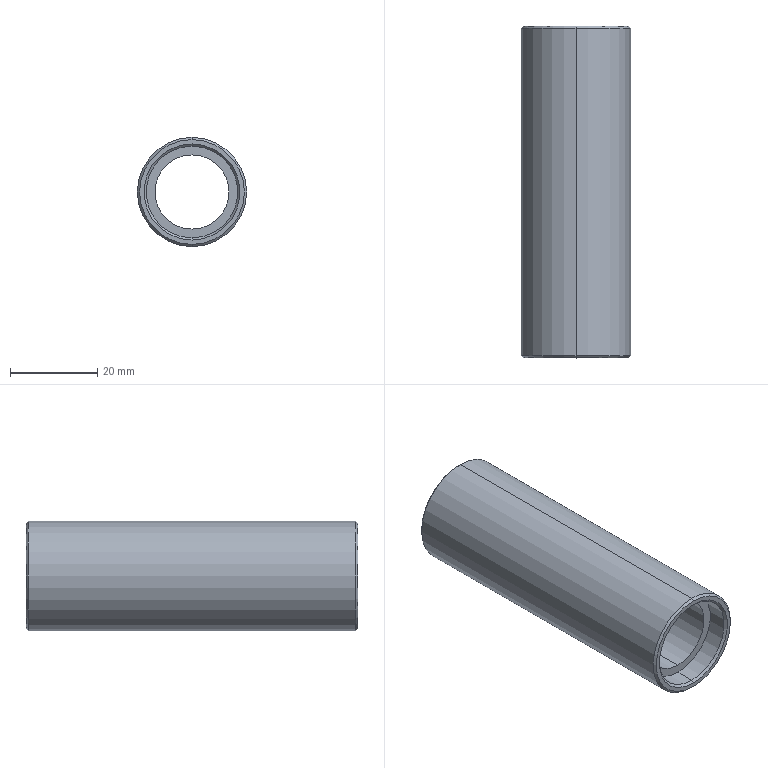Part | STEP file | 10000020451swp000-1 | 1 solid | 20 faces | box 25 x 76 x 25 mm | volume 18826 mm3 | cone 8 | cylinder 8 | plane 4 | commonest cylinder face diameters 21 x4 17 x2 25 x2
STEP:
#1=CARTESIAN_POINT('',(0.,76.,12.));
#2=VERTEX_POINT('',#1);
#3=CARTESIAN_POINT('',(0.,76.,-12.));
#4=VERTEX_POINT('',#3);
#5=CARTESIAN_POINT('',(0.,76.,0.));
#6=DIRECTION('',(0.,1.,0.));
#7=DIRECTION('',(0.,0.,1.));
#8=AXIS2_PLACEMENT_3D('',#5,#6,#7);
#9=CIRCLE('',#8,12.);
#10=EDGE_CURVE('',#2,#4,#9,.T.);
#11=ORIENTED_EDGE('',*,*,#10,.F.);
#12=CARTESIAN_POINT('',(0.,75.5,12.5));
#13=VERTEX_POINT('',#12);
#14=CARTESIAN_POINT('',(0.,76.,12.));
#15=DIRECTION('',(0.,-0.7071,0.7071));
#16=VECTOR('',#15,1000.);
#17=LINE('',#14,#16);
#18=EDGE_CURVE('',#2,#13,#17,.T.);
#19=ORIENTED_EDGE('',*,*,#18,.T.);
#20=CARTESIAN_POINT('',(0.,75.5,-12.5));
#21=VERTEX_POINT('',#20);
#22=CARTESIAN_POINT('',(0.,75.5,0.));
#23=DIRECTION('',(0.,-1.,0.));
#24=DIRECTION('',(0.,0.,1.));
#25=AXIS2_PLACEMENT_3D('',#22,#23,#24);
#26=CIRCLE('',#25,12.5);
#27=EDGE_CURVE('',#21,#13,#26,.T.);
#28=ORIENTED_EDGE('',*,*,#27,.F.);
#29=CARTESIAN_POINT('',(0.,76.,-12.));
#30=DIRECTION('',(0.,-0.7071,-0.7071));
#31=VECTOR('',#30,1000.);
#32=LINE('',#29,#31);
#33=EDGE_CURVE('',#4,#21,#32,.T.);
#34=ORIENTED_EDGE('',*,*,#33,.F.);
#35=EDGE_LOOP('',(#11,#19,#28,#34));
#36=FACE_OUTER_BOUND('',#35,.T.);
#37=CARTESIAN_POINT('',(0.,76.,0.));
#38=DIRECTION('',(0.,-1.,0.));
#39=DIRECTION('',(0.,0.,-1.));
#40=AXIS2_PLACEMENT_3D('',#37,#38,#39);
#41=CONICAL_SURFACE('',#40,12.,0.7854);
#42=ADVANCED_FACE('',(#36),#41,.T.);
#43=CARTESIAN_POINT('',(0.,75.5,-10.5));
#44=VERTEX_POINT('',#43);
#45=CARTESIAN_POINT('',(0.,75.5,10.5));
#46=VERTEX_POINT('',#45);
#47=CARTESIAN_POINT('',(0.,75.5,0.));
#48=DIRECTION('',(0.,1.,0.));
#49=DIRECTION('',(0.,0.,1.));
#50=AXIS2_PLACEMENT_3D('',#47,#48,#49);
#51=CIRCLE('',#50,10.5);
#52=EDGE_CURVE('',#44,#46,#51,.T.);
#53=ORIENTED_EDGE('',*,*,#52,.F.);
#54=CARTESIAN_POINT('',(0.,76.,-11.));
#55=VERTEX_POINT('',#54);
#56=CARTESIAN_POINT('',(0.,75.5,-10.5));
#57=DIRECTION('',(0.,0.7071,-0.7071));
#58=VECTOR('',#57,1000.);
#59=LINE('',#56,#58);
#60=EDGE_CURVE('',#44,#55,#59,.T.);
#61=ORIENTED_EDGE('',*,*,#60,.T.);
#62=CARTESIAN_POINT('',(0.,76.,11.));
#63=VERTEX_POINT('',#62);
#64=CARTESIAN_POINT('',(0.,76.,0.));
#65=DIRECTION('',(0.,-1.,0.));
#66=DIRECTION('',(0.,0.,1.));
#67=AXIS2_PLACEMENT_3D('',#64,#65,#66);
#68=CIRCLE('',#67,11.);
#69=EDGE_CURVE('',#63,#55,#68,.T.);
#70=ORIENTED_EDGE('',*,*,#69,.F.);
#71=CARTESIAN_POINT('',(0.,75.5,10.5));
#72=DIRECTION('',(0.,0.7071,0.7071));
#73=VECTOR('',#72,1000.);
#74=LINE('',#71,#73);
#75=EDGE_CURVE('',#46,#63,#74,.T.);
#76=ORIENTED_EDGE('',*,*,#75,.F.);
#77=EDGE_LOOP('',(#53,#61,#70,#76));
#78=FACE_OUTER_BOUND('',#77,.T.);
#79=CARTESIAN_POINT('',(0.,75.5,0.));
#80=DIRECTION('',(0.,1.,0.));
#81=DIRECTION('',(0.,0.,1.));
#82=AXIS2_PLACEMENT_3D('',#79,#80,#81);
#83=CONICAL_SURFACE('',#82,10.5,0.7854);
#84=ADVANCED_FACE('',(#78),#83,.F.);
#85=CARTESIAN_POINT('',(0.,0.5,10.5));
#86=VERTEX_POINT('',#85);
#87=CARTESIAN_POINT('',(0.,0.5,-10.5));
#88=VERTEX_POINT('',#87);
#89=CARTESIAN_POINT('',(0.,0.5,0.));
#90=DIRECTION('',(0.,-1.,0.));
#91=DIRECTION('',(0.,0.,1.));
#92=AXIS2_PLACEMENT_3D('',#89,#90,#91);
#93=CIRCLE('',#92,10.5);
#94=EDGE_CURVE('',#86,#88,#93,.T.);
#95=ORIENTED_EDGE('',*,*,#94,.F.);
#96=CARTESIAN_POINT('',(0.,0.,11.));
#97=VERTEX_POINT('',#96);
#98=CARTESIAN_POINT('',(0.,0.5,10.5));
#99=DIRECTION('',(0.,-0.7071,0.7071));
#100=VECTOR('',#99,1000.);
#101=LINE('',#98,#100);
#102=EDGE_CURVE('',#86,#97,#101,.T.);
#103=ORIENTED_EDGE('',*,*,#102,.T.);
#104=CARTESIAN_POINT('',(0.,0.,-11.));
#105=VERTEX_POINT('',#104);
#106=CARTESIAN_POINT('',(0.,0.,0.));
#107=DIRECTION('',(0.,1.,0.));
#108=DIRECTION('',(0.,0.,1.));
#109=AXIS2_PLACEMENT_3D('',#106,#107,#108);
#110=CIRCLE('',#109,11.);
#111=EDGE_CURVE('',#105,#97,#110,.T.);
#112=ORIENTED_EDGE('',*,*,#111,.F.);
#113=CARTESIAN_POINT('',(0.,0.5,-10.5));
#114=DIRECTION('',(0.,-0.7071,-0.7071));
#115=VECTOR('',#114,1000.);
#116=LINE('',#113,#115);
#117=EDGE_CURVE('',#88,#105,#116,.T.);
#118=ORIENTED_EDGE('',*,*,#117,.F.);
#119=EDGE_LOOP('',(#95,#103,#112,#118));
#120=FACE_OUTER_BOUND('',#119,.T.);
#121=CARTESIAN_POINT('',(0.,0.5,0.));
#122=DIRECTION('',(0.,-1.,0.));
#123=DIRECTION('',(0.,0.,-1.));
#124=AXIS2_PLACEMENT_3D('',#121,#122,#123);
#125=CONICAL_SURFACE('',#124,10.5,0.7854);
#126=ADVANCED_FACE('',(#120),#125,.F.);
#127=CARTESIAN_POINT('',(0.,0.,-12.));
#128=VERTEX_POINT('',#127);
#129=CARTESIAN_POINT('',(0.,0.,12.));
#130=VERTEX_POINT('',#129);
#131=CARTESIAN_POINT('',(0.,0.,0.));
#132=DIRECTION('',(0.,-1.,0.));
#133=DIRECTION('',(0.,0.,1.));
#134=AXIS2_PLACEMENT_3D('',#131,#132,#133);
#135=CIRCLE('',#134,12.);
#136=EDGE_CURVE('',#128,#130,#135,.T.);
#137=ORIENTED_EDGE('',*,*,#136,.F.);
#138=CARTESIAN_POINT('',(0.,0.5,-12.5));
#139=VERTEX_POINT('',#138);
#140=CARTESIAN_POINT('',(0.,0.5,-12.5));
#141=DIRECTION('',(0.,0.7071,-0.7071));
#142=VECTOR('',#141,1000.);
#143=LINE('',#140,#142);
#144=EDGE_CURVE('',#128,#139,#143,.T.);
#145=ORIENTED_EDGE('',*,*,#144,.T.);
#146=CARTESIAN_POINT('',(0.,0.5,12.5));
#147=VERTEX_POINT('',#146);
#148=CARTESIAN_POINT('',(0.,0.5,0.));
#149=DIRECTION('',(0.,1.,0.));
#150=DIRECTION('',(0.,0.,1.));
#151=AXIS2_PLACEMENT_3D('',#148,#149,#150);
#152=CIRCLE('',#151,12.5);
#153=EDGE_CURVE('',#147,#139,#152,.T.);
#154=ORIENTED_EDGE('',*,*,#153,.F.);
#155=CARTESIAN_POINT('',(0.,0.5,12.5));
#156=DIRECTION('',(0.,0.7071,0.7071));
#157=VECTOR('',#156,1000.);
#158=LINE('',#155,#157);
#159=EDGE_CURVE('',#130,#147,#158,.T.);
#160=ORIENTED_EDGE('',*,*,#159,.F.);
#161=EDGE_LOOP('',(#137,#145,#154,#160));
#162=FACE_OUTER_BOUND('',#161,.T.);
#163=CARTESIAN_POINT('',(0.,0.5,0.));
#164=DIRECTION('',(0.,1.,0.));
#165=DIRECTION('',(0.,0.,1.));
#166=AXIS2_PLACEMENT_3D('',#163,#164,#165);
#167=CONICAL_SURFACE('',#166,12.5,0.7854);
#168=ADVANCED_FACE('',(#162),#167,.T.);
#169=CARTESIAN_POINT('',(0.,71.,-10.5));
#170=VERTEX_POINT('',#169);
#171=CARTESIAN_POINT('',(0.,71.,10.5));
#172=VERTEX_POINT('',#171);
#173=CARTESIAN_POINT('',(0.,71.,0.));
#174=DIRECTION('',(0.,1.,0.));
#175=DIRECTION('',(0.,0.,1.));
#176=AXIS2_PLACEMENT_3D('',#173,#174,#175);
#177=CIRCLE('',#176,10.5);
#178=EDGE_CURVE('',#170,#172,#177,.T.);
#179=ORIENTED_EDGE('',*,*,#178,.F.);
#180=CARTESIAN_POINT('',(0.,76.,-10.5));
#181=DIRECTION('',(0.,1.,0.));
#182=VECTOR('',#181,1000.);
#183=LINE('',#180,#182);
#184=EDGE_CURVE('',#170,#44,#183,.T.);
#185=ORIENTED_EDGE('',*,*,#184,.T.);
#186=ORIENTED_EDGE('',*,*,#52,.T.);
#187=CARTESIAN_POINT('',(0.,76.,10.5));
#188=DIRECTION('',(0.,1.,0.));
#189=VECTOR('',#188,1000.);
#190=LINE('',#187,#189);
#191=EDGE_CURVE('',#172,#46,#190,.T.);
#192=ORIENTED_EDGE('',*,*,#191,.F.);
#193=EDGE_LOOP('',(#179,#185,#186,#192));
#194=FACE_OUTER_BOUND('',#193,.T.);
#195=CARTESIAN_POINT('',(0.,76.,0.));
#196=DIRECTION('',(0.,1.,0.));
#197=DIRECTION('',(0.,0.,1.));
#198=AXIS2_PLACEMENT_3D('',#195,#196,#197);
#199=CYLINDRICAL_SURFACE('',#198,10.5);
#200=ADVANCED_FACE('',(#194),#199,.F.);
#201=CARTESIAN_POINT('',(0.,5.,10.5));
#202=VERTEX_POINT('',#201);
#203=CARTESIAN_POINT('',(0.,5.,-10.5));
#204=VERTEX_POINT('',#203);
#205=CARTESIAN_POINT('',(0.,5.,0.));
#206=DIRECTION('',(0.,-1.,0.));
#207=DIRECTION('',(0.,0.,-1.));
#208=AXIS2_PLACEMENT_3D('',#205,#206,#207);
#209=CIRCLE('',#208,10.5);
#210=EDGE_CURVE('',#202,#204,#209,.T.);
#211=ORIENTED_EDGE('',*,*,#210,.F.);
#212=CARTESIAN_POINT('',(0.,0.,10.5));
#213=DIRECTION('',(0.,-1.,0.));
#214=VECTOR('',#213,1000.);
#215=LINE('',#212,#214);
#216=EDGE_CURVE('',#202,#86,#215,.T.);
#217=ORIENTED_EDGE('',*,*,#216,.T.);
#218=ORIENTED_EDGE('',*,*,#94,.T.);
#219=CARTESIAN_POINT('',(0.,0.,-10.5));
#220=DIRECTION('',(0.,-1.,0.));
#221=VECTOR('',#220,1000.);
#222=LINE('',#219,#221);
#223=EDGE_CURVE('',#204,#88,#222,.T.);
#224=ORIENTED_EDGE('',*,*,#223,.F.);
#225=EDGE_LOOP('',(#211,#217,#218,#224));
#226=FACE_OUTER_BOUND('',#225,.T.);
#227=CARTESIAN_POINT('',(0.,0.,0.));
#228=DIRECTION('',(0.,-1.,0.));
#229=DIRECTION('',(0.,0.,-1.));
#230=AXIS2_PLACEMENT_3D('',#227,#228,#229);
#231=CYLINDRICAL_SURFACE('',#230,10.5);
#232=ADVANCED_FACE('',(#226),#231,.F.);
#233=CARTESIAN_POINT('',(0.,71.,8.5));
#234=VERTEX_POINT('',#233);
#235=CARTESIAN_POINT('',(0.,71.,-8.5));
#236=VERTEX_POINT('',#235);
#237=CARTESIAN_POINT('',(0.,71.,0.));
#238=DIRECTION('',(0.,-1.,0.));
#239=DIRECTION('',(0.,0.,-1.));
#240=AXIS2_PLACEMENT_3D('',#237,#238,#239);
#241=CIRCLE('',#240,8.5);
#242=EDGE_CURVE('',#234,#236,#241,.T.);
#243=ORIENTED_EDGE('',*,*,#242,.F.);
#244=CARTESIAN_POINT('',(0.,5.,8.5));
#245=VERTEX_POINT('',#244);
#246=CARTESIAN_POINT('',(0.,76.,8.5));
#247=DIRECTION('',(0.,-1.,0.));
#248=VECTOR('',#247,1000.);
#249=LINE('',#246,#248);
#250=EDGE_CURVE('',#234,#245,#249,.T.);
#251=ORIENTED_EDGE('',*,*,#250,.T.);
#252=CARTESIAN_POINT('',(0.,5.,-8.5));
#253=VERTEX_POINT('',#252);
#254=CARTESIAN_POINT('',(0.,5.,0.));
#255=DIRECTION('',(0.,1.,0.));
#256=DIRECTION('',(0.,0.,1.));
#257=AXIS2_PLACEMENT_3D('',#254,#255,#256);
#258=CIRCLE('',#257,8.5);
#259=EDGE_CURVE('',#253,#245,#258,.T.);
#260=ORIENTED_EDGE('',*,*,#259,.F.);
#261=CARTESIAN_POINT('',(0.,76.,-8.5));
#262=DIRECTION('',(0.,-1.,0.));
#263=VECTOR('',#262,1000.);
#264=LINE('',#261,#263);
#265=EDGE_CURVE('',#236,#253,#264,.T.);
#266=ORIENTED_EDGE('',*,*,#265,.F.);
#267=EDGE_LOOP('',(#243,#251,#260,#266));
#268=FACE_OUTER_BOUND('',#267,.T.);
#269=CARTESIAN_POINT('',(0.,76.,0.));
#270=DIRECTION('',(0.,-1.,0.));
#271=DIRECTION('',(0.,0.,-1.));
#272=AXIS2_PLACEMENT_3D('',#269,#270,#271);
#273=CYLINDRICAL_SURFACE('',#272,8.5);
#274=ADVANCED_FACE('',(#268),#273,.F.);
#275=ORIENTED_EDGE('',*,*,#27,.T.);
#276=CARTESIAN_POINT('',(0.,76.,12.5));
#277=DIRECTION('',(0.,-1.,0.));
#278=VECTOR('',#277,1000.);
#279=LINE('',#276,#278);
#280=EDGE_CURVE('',#13,#147,#279,.T.);
#281=ORIENTED_EDGE('',*,*,#280,.T.);
#282=ORIENTED_EDGE('',*,*,#153,.T.);
#283=CARTESIAN_POINT('',(0.,76.,-12.5));
#284=DIRECTION('',(0.,-1.,0.));
#285=VECTOR('',#284,1000.);
#286=LINE('',#283,#285);
#287=EDGE_CURVE('',#21,#139,#286,.T.);
#288=ORIENTED_EDGE('',*,*,#287,.F.);
#289=EDGE_LOOP('',(#275,#281,#282,#288));
#290=FACE_OUTER_BOUND('',#289,.T.);
#291=CARTESIAN_POINT('',(0.,76.,0.));
#292=DIRECTION('',(0.,-1.,0.));
#293=DIRECTION('',(0.,0.,-1.));
#294=AXIS2_PLACEMENT_3D('',#291,#292,#293);
#295=CYLINDRICAL_SURFACE('',#294,12.5);
#296=ADVANCED_FACE('',(#290),#295,.T.);
#297=ORIENTED_EDGE('',*,*,#69,.T.);
#298=CARTESIAN_POINT('',(0.,76.,0.));
#299=DIRECTION('',(0.,-1.,0.));
#300=DIRECTION('',(0.,0.,1.));
#301=AXIS2_PLACEMENT_3D('',#298,#299,#300);
#302=CIRCLE('',#301,11.);
#303=EDGE_CURVE('',#55,#63,#302,.T.);
#304=ORIENTED_EDGE('',*,*,#303,.T.);
#305=EDGE_LOOP('',(#297,#304));
#306=FACE_BOUND('',#305,.T.);
#307=CARTESIAN_POINT('',(0.,76.,0.));
#308=DIRECTION('',(0.,1.,0.));
#309=DIRECTION('',(0.,0.,1.));
#310=AXIS2_PLACEMENT_3D('',#307,#308,#309);
#311=CIRCLE('',#310,12.);
#312=EDGE_CURVE('',#4,#2,#311,.T.);
#313=ORIENTED_EDGE('',*,*,#312,.T.);
#314=ORIENTED_EDGE('',*,*,#10,.T.);
#315=EDGE_LOOP('',(#313,#314));
#316=FACE_OUTER_BOUND('',#315,.T.);
#317=CARTESIAN_POINT('',(0.,76.,0.));
#318=DIRECTION('',(0.,1.,0.));
#319=DIRECTION('',(0.,0.,1.));
#320=AXIS2_PLACEMENT_3D('',#317,#318,#319);
#321=PLANE('',#320);
#322=ADVANCED_FACE('',(#306,#316),#321,.T.);
#323=CARTESIAN_POINT('',(0.,0.,0.));
#324=DIRECTION('',(0.,-1.,0.));
#325=DIRECTION('',(0.,0.,1.));
#326=AXIS2_PLACEMENT_3D('',#323,#324,#325);
#327=CIRCLE('',#326,12.);
#328=EDGE_CURVE('',#130,#128,#327,.T.);
#329=ORIENTED_EDGE('',*,*,#328,.T.);
#330=ORIENTED_EDGE('',*,*,#136,.T.);
#331=EDGE_LOOP('',(#329,#330));
#332=FACE_OUTER_BOUND('',#331,.T.);
#333=ORIENTED_EDGE('',*,*,#111,.T.);
#334=CARTESIAN_POINT('',(0.,0.,0.));
#335=DIRECTION('',(0.,1.,0.));
#336=DIRECTION('',(0.,0.,1.));
#337=AXIS2_PLACEMENT_3D('',#334,#335,#336);
#338=CIRCLE('',#337,11.);
#339=EDGE_CURVE('',#97,#105,#338,.T.);
#340=ORIENTED_EDGE('',*,*,#339,.T.);
#341=EDGE_LOOP('',(#333,#340));
#342=FACE_BOUND('',#341,.T.);
#343=CARTESIAN_POINT('',(0.,0.,0.));
#344=DIRECTION('',(0.,1.,0.));
#345=DIRECTION('',(0.,0.,1.));
#346=AXIS2_PLACEMENT_3D('',#343,#344,#345);
#347=PLANE('',#346);
#348=ADVANCED_FACE('',(#332,#342),#347,.F.);
#349=ORIENTED_EDGE('',*,*,#280,.F.);
#350=CARTESIAN_POINT('',(0.,75.5,0.));
#351=DIRECTION('',(0.,-1.,0.));
#352=DIRECTION('',(0.,0.,1.));
#353=AXIS2_PLACEMENT_3D('',#350,#351,#352);
#354=CIRCLE('',#353,12.5);
#355=EDGE_CURVE('',#13,#21,#354,.T.);
#356=ORIENTED_EDGE('',*,*,#355,.T.);
#357=ORIENTED_EDGE('',*,*,#287,.T.);
#358=CARTESIAN_POINT('',(0.,0.5,0.));
#359=DIRECTION('',(0.,1.,0.));
#360=DIRECTION('',(0.,0.,1.));
#361=AXIS2_PLACEMENT_3D('',#358,#359,#360);
#362=CIRCLE('',#361,12.5);
#363=EDGE_CURVE('',#139,#147,#362,.T.);
#364=ORIENTED_EDGE('',*,*,#363,.T.);
#365=EDGE_LOOP('',(#349,#356,#357,#364));
#366=FACE_OUTER_BOUND('',#365,.T.);
#367=CARTESIAN_POINT('',(0.,76.,0.));
#368=DIRECTION('',(0.,-1.,0.));
#369=DIRECTION('',(0.,0.,-1.));
#370=AXIS2_PLACEMENT_3D('',#367,#368,#369);
#371=CYLINDRICAL_SURFACE('',#370,12.5);
#372=ADVANCED_FACE('',(#366),#371,.T.);
#373=ORIENTED_EDGE('',*,*,#250,.F.);
#374=CARTESIAN_POINT('',(0.,71.,0.));
#375=DIRECTION('',(0.,-1.,0.));
#376=DIRECTION('',(0.,0.,-1.));
#377=AXIS2_PLACEMENT_3D('',#374,#375,#376);
#378=CIRCLE('',#377,8.5);
#379=EDGE_CURVE('',#236,#234,#378,.T.);
#380=ORIENTED_EDGE('',*,*,#379,.F.);
#381=ORIENTED_EDGE('',*,*,#265,.T.);
#382=CARTESIAN_POINT('',(0.,5.,0.));
#383=DIRECTION('',(0.,1.,0.));
#384=DIRECTION('',(0.,0.,1.));
#385=AXIS2_PLACEMENT_3D('',#382,#383,#384);
#386=CIRCLE('',#385,8.5);
#387=EDGE_CURVE('',#245,#253,#386,.T.);
#388=ORIENTED_EDGE('',*,*,#387,.F.);
#389=EDGE_LOOP('',(#373,#380,#381,#388));
#390=FACE_OUTER_BOUND('',#389,.T.);
#391=CARTESIAN_POINT('',(0.,76.,0.));
#392=DIRECTION('',(0.,-1.,0.));
#393=DIRECTION('',(0.,0.,-1.));
#394=AXIS2_PLACEMENT_3D('',#391,#392,#393);
#395=CYLINDRICAL_SURFACE('',#394,8.5);
#396=ADVANCED_FACE('',(#390),#395,.F.);
#397=ORIENTED_EDGE('',*,*,#259,.T.);
#398=ORIENTED_EDGE('',*,*,#387,.T.);
#399=EDGE_LOOP('',(#397,#398));
#400=FACE_BOUND('',#399,.T.);
#401=CARTESIAN_POINT('',(0.,5.,0.));
#402=DIRECTION('',(0.,-1.,0.));
#403=DIRECTION('',(0.,0.,-1.));
#404=AXIS2_PLACEMENT_3D('',#401,#402,#403);
#405=CIRCLE('',#404,10.5);
#406=EDGE_CURVE('',#204,#202,#405,.T.);
#407=ORIENTED_EDGE('',*,*,#406,.T.);
#408=ORIENTED_EDGE('',*,*,#210,.T.);
#409=EDGE_LOOP('',(#407,#408));
#410=FACE_OUTER_BOUND('',#409,.T.);
#411=CARTESIAN_POINT('',(0.,5.,0.));
#412=DIRECTION('',(0.,1.,0.));
#413=DIRECTION('',(0.,0.,1.));
#414=AXIS2_PLACEMENT_3D('',#411,#412,#413);
#415=PLANE('',#414);
#416=ADVANCED_FACE('',(#400,#410),#415,.F.);
#417=ORIENTED_EDGE('',*,*,#216,.F.);
#418=ORIENTED_EDGE('',*,*,#406,.F.);
#419=ORIENTED_EDGE('',*,*,#223,.T.);
#420=CARTESIAN_POINT('',(0.,0.5,0.));
#421=DIRECTION('',(0.,-1.,0.));
#422=DIRECTION('',(0.,0.,1.));
#423=AXIS2_PLACEMENT_3D('',#420,#421,#422);
#424=CIRCLE('',#423,10.5);
#425=EDGE_CURVE('',#88,#86,#424,.T.);
#426=ORIENTED_EDGE('',*,*,#425,.T.);
#427=EDGE_LOOP('',(#417,#418,#419,#426));
#428=FACE_OUTER_BOUND('',#427,.T.);
#429=CARTESIAN_POINT('',(0.,0.,0.));
#430=DIRECTION('',(0.,-1.,0.));
#431=DIRECTION('',(0.,0.,-1.));
#432=AXIS2_PLACEMENT_3D('',#429,#430,#431);
#433=CYLINDRICAL_SURFACE('',#432,10.5);
#434=ADVANCED_FACE('',(#428),#433,.F.);
#435=ORIENTED_EDGE('',*,*,#379,.T.);
#436=ORIENTED_EDGE('',*,*,#242,.T.);
#437=EDGE_LOOP('',(#435,#436));
#438=FACE_BOUND('',#437,.T.);
#439=CARTESIAN_POINT('',(0.,71.,0.));
#440=DIRECTION('',(0.,1.,0.));
#441=DIRECTION('',(0.,0.,1.));
#442=AXIS2_PLACEMENT_3D('',#439,#440,#441);
#443=CIRCLE('',#442,10.5);
#444=EDGE_CURVE('',#172,#170,#443,.T.);
#445=ORIENTED_EDGE('',*,*,#444,.T.);
#446=ORIENTED_EDGE('',*,*,#178,.T.);
#447=EDGE_LOOP('',(#445,#446));
#448=FACE_OUTER_BOUND('',#447,.T.);
#449=CARTESIAN_POINT('',(0.,71.,0.));
#450=DIRECTION('',(0.,-1.,0.));
#451=DIRECTION('',(0.,0.,-1.));
#452=AXIS2_PLACEMENT_3D('',#449,#450,#451);
#453=PLANE('',#452);
#454=ADVANCED_FACE('',(#438,#448),#453,.F.);
#455=ORIENTED_EDGE('',*,*,#184,.F.);
#456=ORIENTED_EDGE('',*,*,#444,.F.);
#457=ORIENTED_EDGE('',*,*,#191,.T.);
#458=CARTESIAN_POINT('',(0.,75.5,0.));
#459=DIRECTION('',(0.,1.,0.));
#460=DIRECTION('',(0.,0.,1.));
#461=AXIS2_PLACEMENT_3D('',#458,#459,#460);
#462=CIRCLE('',#461,10.5);
#463=EDGE_CURVE('',#46,#44,#462,.T.);
#464=ORIENTED_EDGE('',*,*,#463,.T.);
#465=EDGE_LOOP('',(#455,#456,#457,#464));
#466=FACE_OUTER_BOUND('',#465,.T.);
#467=CARTESIAN_POINT('',(0.,76.,0.));
#468=DIRECTION('',(0.,1.,0.));
#469=DIRECTION('',(0.,0.,1.));
#470=AXIS2_PLACEMENT_3D('',#467,#468,#469);
#471=CYLINDRICAL_SURFACE('',#470,10.5);
#472=ADVANCED_FACE('',(#466),#471,.F.);
#473=ORIENTED_EDGE('',*,*,#144,.F.);
#474=ORIENTED_EDGE('',*,*,#328,.F.);
#475=ORIENTED_EDGE('',*,*,#159,.T.);
#476=ORIENTED_EDGE('',*,*,#363,.F.);
#477=EDGE_LOOP('',(#473,#474,#475,#476));
#478=FACE_OUTER_BOUND('',#477,.T.);
#479=CARTESIAN_POINT('',(0.,0.5,0.));
#480=DIRECTION('',(0.,1.,0.));
#481=DIRECTION('',(0.,0.,1.));
#482=AXIS2_PLACEMENT_3D('',#479,#480,#481);
#483=CONICAL_SURFACE('',#482,12.5,0.7854);
#484=ADVANCED_FACE('',(#478),#483,.T.);
#485=ORIENTED_EDGE('',*,*,#102,.F.);
#486=ORIENTED_EDGE('',*,*,#425,.F.);
#487=ORIENTED_EDGE('',*,*,#117,.T.);
#488=ORIENTED_EDGE('',*,*,#339,.F.);
#489=EDGE_LOOP('',(#485,#486,#487,#488));
#490=FACE_OUTER_BOUND('',#489,.T.);
#491=CARTESIAN_POINT('',(0.,0.5,0.));
#492=DIRECTION('',(0.,-1.,0.));
#493=DIRECTION('',(0.,0.,-1.));
#494=AXIS2_PLACEMENT_3D('',#491,#492,#493);
#495=CONICAL_SURFACE('',#494,10.5,0.7854);
#496=ADVANCED_FACE('',(#490),#495,.F.);
#497=ORIENTED_EDGE('',*,*,#60,.F.);
#498=ORIENTED_EDGE('',*,*,#463,.F.);
#499=ORIENTED_EDGE('',*,*,#75,.T.);
#500=ORIENTED_EDGE('',*,*,#303,.F.);
#501=EDGE_LOOP('',(#497,#498,#499,#500));
#502=FACE_OUTER_BOUND('',#501,.T.);
#503=CARTESIAN_POINT('',(0.,75.5,0.));
#504=DIRECTION('',(0.,1.,0.));
#505=DIRECTION('',(0.,0.,1.));
#506=AXIS2_PLACEMENT_3D('',#503,#504,#505);
#507=CONICAL_SURFACE('',#506,10.5,0.7854);
#508=ADVANCED_FACE('',(#502),#507,.F.);
#509=ORIENTED_EDGE('',*,*,#18,.F.);
#510=ORIENTED_EDGE('',*,*,#312,.F.);
#511=ORIENTED_EDGE('',*,*,#33,.T.);
#512=ORIENTED_EDGE('',*,*,#355,.F.);
#513=EDGE_LOOP('',(#509,#510,#511,#512));
#514=FACE_OUTER_BOUND('',#513,.T.);
#515=CARTESIAN_POINT('',(0.,76.,0.));
#516=DIRECTION('',(0.,-1.,0.));
#517=DIRECTION('',(0.,0.,-1.));
#518=AXIS2_PLACEMENT_3D('',#515,#516,#517);
#519=CONICAL_SURFACE('',#518,12.,0.7854);
#520=ADVANCED_FACE('',(#514),#519,.T.);
#521=CLOSED_SHELL('',(#42,#84,#126,#168,#200,#232,#274,#296,#322,#348,#372,#396,#416,#434,#454,#472,#484,#496,#508,#520));
#522=MANIFOLD_SOLID_BREP('',#521);
#523=CARTESIAN_POINT('',(0.,0.,0.));
#524=DIRECTION('',(0.,0.,1.));
#525=DIRECTION('',(1.,0.,0.));
#526=AXIS2_PLACEMENT_3D('',#523,#524,#525);
#527=(LENGTH_UNIT()NAMED_UNIT(*)SI_UNIT(.MILLI.,.METRE.));
#528=UNCERTAINTY_MEASURE_WITH_UNIT(LENGTH_MEASURE(0.00001),#527,'','');
#529=(NAMED_UNIT(*)PLANE_ANGLE_UNIT()SI_UNIT($,.RADIAN.));
#530=(NAMED_UNIT(*)SI_UNIT($,.STERADIAN.)SOLID_ANGLE_UNIT());
#531=(GEOMETRIC_REPRESENTATION_CONTEXT(3)GLOBAL_UNCERTAINTY_ASSIGNED_CONTEXT((#528))GLOBAL_UNIT_ASSIGNED_CONTEXT((#527,#529,#530))REPRESENTATION_CONTEXT('',''));
#532=ADVANCED_BREP_SHAPE_REPRESENTATION('',(#522,#526),#531);